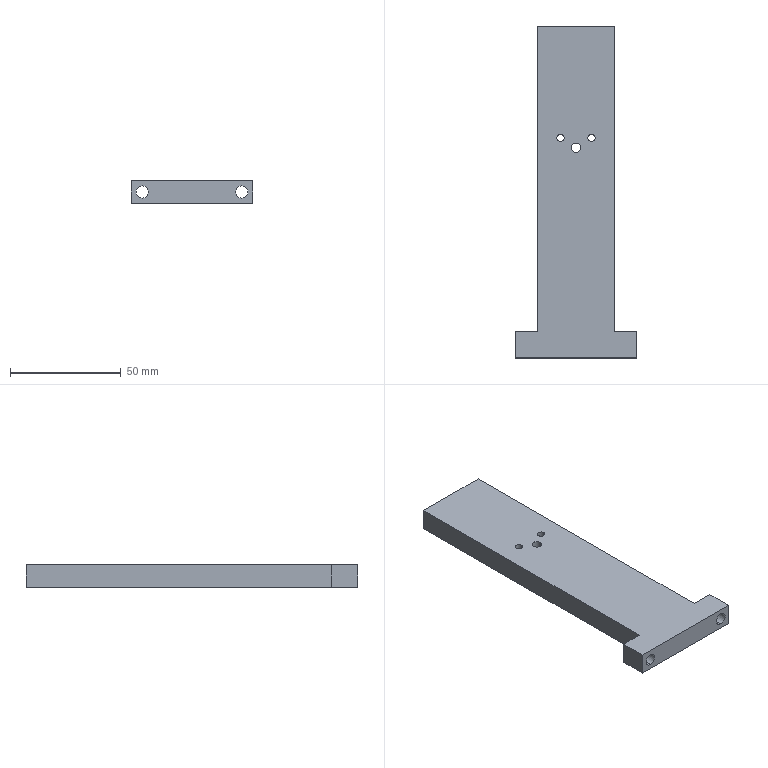Part | STEP file | D07 | 1 solid | 28 faces | box 55 x 150 x 10 mm | volume 53842 mm3 | cylinder 14 | plane 10 | cone 4 | commonest cylinder face diameters 3.3 x8 5.5 x4 4.2 x2